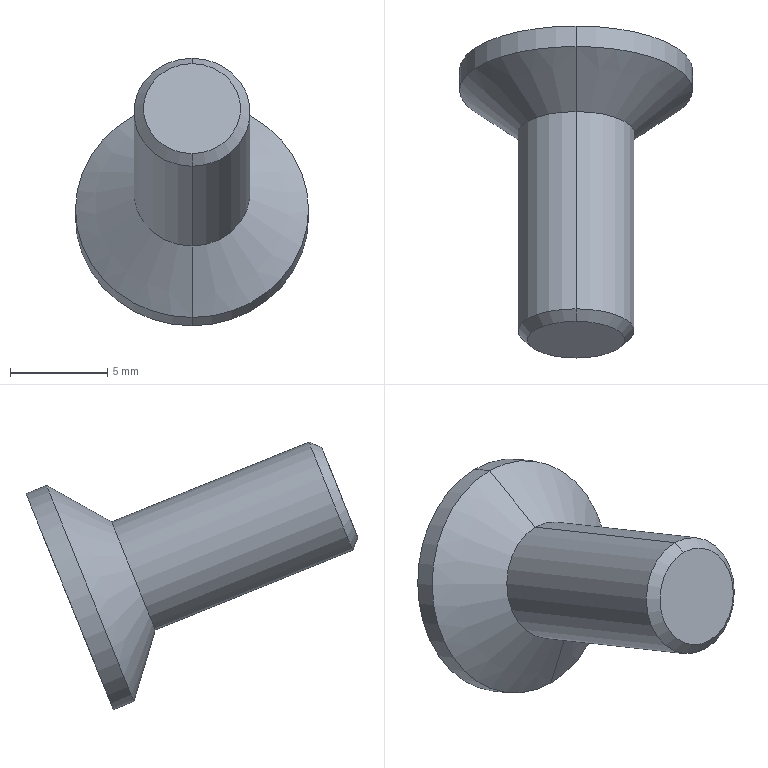Part | Creo | 1 solid | 18 faces | box 12 x 17.092 x 13.776 mm | volume 560.254 mm3 | plane 8 | cone 6 | cylinder 4 | commonest cylinder face diameters 6 x2 12 x2
STEP:
#1=CARTESIAN_POINT('',(50.258,-269.39,4.596));
#2=VERTEX_POINT('',#1);
#3=CARTESIAN_POINT('',(52.258,-269.822,3.525));
#4=VERTEX_POINT('',#3);
#5=CARTESIAN_POINT('',(50.258,-269.39,4.596));
#6=CARTESIAN_POINT('',(50.351,-269.439,4.558));
#7=CARTESIAN_POINT('',(50.539,-269.531,4.479));
#8=CARTESIAN_POINT('',(50.825,-269.649,4.348));
#9=CARTESIAN_POINT('',(51.114,-269.742,4.205));
#10=CARTESIAN_POINT('',(51.404,-269.804,4.05));
#11=CARTESIAN_POINT('',(51.693,-269.837,3.883));
#12=CARTESIAN_POINT('',(51.979,-269.842,3.707));
#13=CARTESIAN_POINT('',(52.166,-269.831,3.587));
#14=CARTESIAN_POINT('',(52.258,-269.822,3.525));
#15=B_SPLINE_CURVE_WITH_KNOTS('',3,(#5,#6,#7,#8,#9,#10,#11,#12,#13,#14),.UNSPECIFIED.,.F.,.F.,(4,1,1,1,1,1,1,4),(0.,0.1429,0.2857,0.4286,0.5714,0.7143,0.8571,1.),.UNSPECIFIED.);
#16=EDGE_CURVE('',#2,#4,#15,.T.);
#17=ORIENTED_EDGE('',*,*,#16,.F.);
#18=CARTESIAN_POINT('',(50.258,-271.491,2.954));
#19=VERTEX_POINT('',#18);
#20=CARTESIAN_POINT('',(50.258,-271.491,2.954));
#21=DIRECTION('',(0.,0.788,0.6157));
#22=VECTOR('',#21,2.667);
#23=LINE('',#20,#22);
#24=EDGE_CURVE('',#19,#2,#23,.T.);
#25=ORIENTED_EDGE('',*,*,#24,.F.);
#26=CARTESIAN_POINT('',(50.258,-271.12,0.3135));
#27=VERTEX_POINT('',#26);
#28=CARTESIAN_POINT('',(50.258,-271.491,2.954));
#29=DIRECTION('',(0.,0.1392,-0.9903));
#30=VECTOR('',#29,2.667);
#31=LINE('',#28,#30);
#32=EDGE_CURVE('',#19,#27,#31,.T.);
#33=ORIENTED_EDGE('',*,*,#32,.T.);
#34=CARTESIAN_POINT('',(52.258,-270.687,1.384));
#35=VERTEX_POINT('',#34);
#36=CARTESIAN_POINT('',(52.258,-270.687,1.384));
#37=CARTESIAN_POINT('',(52.166,-270.736,1.346));
#38=CARTESIAN_POINT('',(51.979,-270.828,1.267));
#39=CARTESIAN_POINT('',(51.693,-270.947,1.137));
#40=CARTESIAN_POINT('',(51.404,-271.039,0.9941));
#41=CARTESIAN_POINT('',(51.114,-271.102,0.8392));
#42=CARTESIAN_POINT('',(50.825,-271.134,0.6724));
#43=CARTESIAN_POINT('',(50.539,-271.14,0.4961));
#44=CARTESIAN_POINT('',(50.351,-271.129,0.375));
#45=CARTESIAN_POINT('',(50.258,-271.12,0.3135));
#46=B_SPLINE_CURVE_WITH_KNOTS('',3,(#36,#37,#38,#39,#40,#41,#42,#43,#44,#45),.UNSPECIFIED.,.F.,.F.,(4,1,1,1,1,1,1,4),(0.,0.1429,0.2857,0.4286,0.5714,0.7143,0.8571,1.),.UNSPECIFIED.);
#47=EDGE_CURVE('',#35,#27,#46,.T.);
#48=ORIENTED_EDGE('',*,*,#47,.F.);
#49=CARTESIAN_POINT('',(52.258,-269.822,3.525));
#50=CARTESIAN_POINT('',(52.258,-269.862,3.474));
#51=CARTESIAN_POINT('',(52.258,-269.939,3.373));
#52=CARTESIAN_POINT('',(52.258,-270.044,3.224));
#53=CARTESIAN_POINT('',(52.258,-270.14,3.075));
#54=CARTESIAN_POINT('',(52.258,-270.229,2.924));
#55=CARTESIAN_POINT('',(52.258,-270.312,2.767));
#56=CARTESIAN_POINT('',(52.258,-270.387,2.605));
#57=CARTESIAN_POINT('',(52.258,-270.454,2.439));
#58=CARTESIAN_POINT('',(52.258,-270.513,2.27));
#59=CARTESIAN_POINT('',(52.258,-270.562,2.1));
#60=CARTESIAN_POINT('',(52.258,-270.603,1.928));
#61=CARTESIAN_POINT('',(52.258,-270.637,1.754));
#62=CARTESIAN_POINT('',(52.258,-270.665,1.575));
#63=CARTESIAN_POINT('',(52.258,-270.681,1.449));
#64=CARTESIAN_POINT('',(52.258,-270.687,1.384));
#65=B_SPLINE_CURVE_WITH_KNOTS('',3,(#49,#50,#51,#52,#53,#54,#55,#56,#57,#58,#59,#60,#61,#62,#63,#64),.UNSPECIFIED.,.F.,.F.,(4,1,1,1,1,1,1,1,1,1,1,1,1,4),(0.,0.07692,0.1538,0.2308,0.3077,0.3846,0.4615,0.5385,0.6154,0.6923,0.7692,0.8462,0.9231,1.),.UNSPECIFIED.);
#66=EDGE_CURVE('',#4,#35,#65,.T.);
#67=ORIENTED_EDGE('',*,*,#66,.F.);
#68=EDGE_LOOP('',(#17,#25,#33,#48,#67));
#69=FACE_OUTER_BOUND('',#68,.F.);
#70=CARTESIAN_POINT('',(50.258,-270.861,2.699));
#71=DIRECTION('',(0.,0.9272,-0.3746));
#72=DIRECTION('',(0.,0.3746,0.9272));
#73=AXIS2_PLACEMENT_3D('',#70,#71,#72);
#74=CONICAL_SURFACE('',#73,1.178,60.);
#75=ADVANCED_FACE('',(#69),#74,.F.);
#76=CARTESIAN_POINT('',(52.258,-267.041,2.402));
#77=VERTEX_POINT('',#76);
#78=CARTESIAN_POINT('',(50.258,-266.608,3.472));
#79=VERTEX_POINT('',#78);
#80=CARTESIAN_POINT('',(52.258,-267.041,2.402));
#81=DIRECTION('',(-0.866,0.1873,0.4636));
#82=VECTOR('',#81,2.309);
#83=LINE('',#80,#82);
#84=EDGE_CURVE('',#77,#79,#83,.T.);
#85=ORIENTED_EDGE('',*,*,#84,.T.);
#86=CARTESIAN_POINT('',(50.258,-266.608,3.472));
#87=DIRECTION('',(0.,-0.9272,0.3746));
#88=VECTOR('',#87,3.);
#89=LINE('',#86,#88);
#90=EDGE_CURVE('',#79,#2,#89,.T.);
#91=ORIENTED_EDGE('',*,*,#90,.T.);
#92=ORIENTED_EDGE('',*,*,#16,.T.);
#93=CARTESIAN_POINT('',(52.258,-267.041,2.402));
#94=DIRECTION('',(0.,-0.9272,0.3746));
#95=VECTOR('',#94,3.);
#96=LINE('',#93,#95);
#97=EDGE_CURVE('',#77,#4,#96,.T.);
#98=ORIENTED_EDGE('',*,*,#97,.F.);
#99=EDGE_LOOP('',(#85,#91,#92,#98));
#100=FACE_OUTER_BOUND('',#99,.F.);
#101=CARTESIAN_POINT('',(50.258,-269.39,4.596));
#102=DIRECTION('',(0.5,0.3244,0.803));
#103=DIRECTION('',(0.866,-0.1873,-0.4636));
#104=AXIS2_PLACEMENT_3D('',#101,#102,#103);
#105=PLANE('',#104);
#106=ADVANCED_FACE('',(#100),#105,.F.);
#107=CARTESIAN_POINT('',(50.258,-265.226,6.894));
#108=VERTEX_POINT('',#107);
#109=CARTESIAN_POINT('',(50.258,-269.721,-4.232));
#110=VERTEX_POINT('',#109);
#111=CARTESIAN_POINT('',(50.258,-267.473,1.331));
#112=DIRECTION('',(0.,0.9272,-0.3746));
#113=DIRECTION('',(0.,0.3746,0.9272));
#114=AXIS2_PLACEMENT_3D('',#111,#112,#113);
#115=CIRCLE('',#114,6.);
#116=EDGE_CURVE('',#108,#110,#115,.T.);
#117=ORIENTED_EDGE('',*,*,#116,.F.);
#118=CARTESIAN_POINT('',(50.258,-267.473,1.331));
#119=DIRECTION('',(0.,0.9272,-0.3746));
#120=DIRECTION('',(0.,-0.3746,-0.9272));
#121=AXIS2_PLACEMENT_3D('',#118,#119,#120);
#122=CIRCLE('',#121,6.);
#123=EDGE_CURVE('',#110,#108,#122,.T.);
#124=ORIENTED_EDGE('',*,*,#123,.F.);
#125=EDGE_LOOP('',(#117,#124));
#126=FACE_OUTER_BOUND('',#125,.F.);
#127=CARTESIAN_POINT('',(52.258,-267.906,0.2603));
#128=VERTEX_POINT('',#127);
#129=CARTESIAN_POINT('',(52.258,-267.906,0.2603));
#130=DIRECTION('',(0.,0.3746,0.9272));
#131=VECTOR('',#130,2.309);
#132=LINE('',#129,#131);
#133=EDGE_CURVE('',#128,#77,#132,.T.);
#134=ORIENTED_EDGE('',*,*,#133,.F.);
#135=CARTESIAN_POINT('',(50.258,-268.338,-0.8103));
#136=VERTEX_POINT('',#135);
#137=CARTESIAN_POINT('',(50.258,-268.338,-0.8103));
#138=DIRECTION('',(0.866,0.1873,0.4636));
#139=VECTOR('',#138,2.309);
#140=LINE('',#137,#139);
#141=EDGE_CURVE('',#136,#128,#140,.T.);
#142=ORIENTED_EDGE('',*,*,#141,.F.);
#143=CARTESIAN_POINT('',(48.258,-267.906,0.2603));
#144=VERTEX_POINT('',#143);
#145=CARTESIAN_POINT('',(48.258,-267.906,0.2603));
#146=DIRECTION('',(0.866,-0.1873,-0.4636));
#147=VECTOR('',#146,2.309);
#148=LINE('',#145,#147);
#149=EDGE_CURVE('',#144,#136,#148,.T.);
#150=ORIENTED_EDGE('',*,*,#149,.F.);
#151=CARTESIAN_POINT('',(48.258,-267.041,2.402));
#152=VERTEX_POINT('',#151);
#153=CARTESIAN_POINT('',(48.258,-267.041,2.402));
#154=DIRECTION('',(0.,-0.3746,-0.9272));
#155=VECTOR('',#154,2.309);
#156=LINE('',#153,#155);
#157=EDGE_CURVE('',#152,#144,#156,.T.);
#158=ORIENTED_EDGE('',*,*,#157,.F.);
#159=CARTESIAN_POINT('',(50.258,-266.608,3.472));
#160=DIRECTION('',(-0.866,-0.1873,-0.4636));
#161=VECTOR('',#160,2.309);
#162=LINE('',#159,#161);
#163=EDGE_CURVE('',#79,#152,#162,.T.);
#164=ORIENTED_EDGE('',*,*,#163,.F.);
#165=ORIENTED_EDGE('',*,*,#84,.F.);
#166=EDGE_LOOP('',(#134,#142,#150,#158,#164,#165));
#167=FACE_BOUND('',#166,.F.);
#168=CARTESIAN_POINT('',(50.258,-265.226,6.894));
#169=DIRECTION('',(0.,-0.9272,0.3746));
#170=DIRECTION('',(0.,-0.3746,-0.9272));
#171=AXIS2_PLACEMENT_3D('',#168,#169,#170);
#172=PLANE('',#171);
#173=ADVANCED_FACE('',(#126,#167),#172,.F.);
#174=ORIENTED_EDGE('',*,*,#133,.T.);
#175=ORIENTED_EDGE('',*,*,#97,.T.);
#176=ORIENTED_EDGE('',*,*,#66,.T.);
#177=CARTESIAN_POINT('',(52.258,-267.906,0.2603));
#178=DIRECTION('',(0.,-0.9272,0.3746));
#179=VECTOR('',#178,3.);
#180=LINE('',#177,#179);
#181=EDGE_CURVE('',#128,#35,#180,.T.);
#182=ORIENTED_EDGE('',*,*,#181,.F.);
#183=EDGE_LOOP('',(#174,#175,#176,#182));
#184=FACE_OUTER_BOUND('',#183,.F.);
#185=CARTESIAN_POINT('',(52.258,-269.822,3.525));
#186=DIRECTION('',(1.,0.,0.));
#187=DIRECTION('',(0.,0.9272,-0.3746));
#188=AXIS2_PLACEMENT_3D('',#185,#186,#187);
#189=PLANE('',#188);
#190=ADVANCED_FACE('',(#184),#189,.F.);
#191=ORIENTED_EDGE('',*,*,#141,.T.);
#192=ORIENTED_EDGE('',*,*,#181,.T.);
#193=ORIENTED_EDGE('',*,*,#47,.T.);
#194=CARTESIAN_POINT('',(50.258,-268.338,-0.8103));
#195=DIRECTION('',(0.,-0.9272,0.3746));
#196=VECTOR('',#195,3.);
#197=LINE('',#194,#196);
#198=EDGE_CURVE('',#136,#27,#197,.T.);
#199=ORIENTED_EDGE('',*,*,#198,.F.);
#200=EDGE_LOOP('',(#191,#192,#193,#199));
#201=FACE_OUTER_BOUND('',#200,.F.);
#202=CARTESIAN_POINT('',(52.258,-270.687,1.384));
#203=DIRECTION('',(0.5,-0.3244,-0.803));
#204=DIRECTION('',(-0.866,-0.1873,-0.4636));
#205=AXIS2_PLACEMENT_3D('',#202,#203,#204);
#206=PLANE('',#205);
#207=ADVANCED_FACE('',(#201),#206,.F.);
#208=ORIENTED_EDGE('',*,*,#149,.T.);
#209=ORIENTED_EDGE('',*,*,#198,.T.);
#210=CARTESIAN_POINT('',(48.258,-270.687,1.384));
#211=VERTEX_POINT('',#210);
#212=CARTESIAN_POINT('',(50.258,-271.12,0.3135));
#213=CARTESIAN_POINT('',(50.165,-271.129,0.375));
#214=CARTESIAN_POINT('',(49.978,-271.14,0.4961));
#215=CARTESIAN_POINT('',(49.692,-271.134,0.6724));
#216=CARTESIAN_POINT('',(49.402,-271.102,0.8392));
#217=CARTESIAN_POINT('',(49.113,-271.039,0.9941));
#218=CARTESIAN_POINT('',(48.824,-270.947,1.137));
#219=CARTESIAN_POINT('',(48.538,-270.828,1.267));
#220=CARTESIAN_POINT('',(48.351,-270.736,1.346));
#221=CARTESIAN_POINT('',(48.258,-270.687,1.384));
#222=B_SPLINE_CURVE_WITH_KNOTS('',3,(#212,#213,#214,#215,#216,#217,#218,#219,#220,#221),.UNSPECIFIED.,.F.,.F.,(4,1,1,1,1,1,1,4),(0.,0.1429,0.2857,0.4286,0.5714,0.7143,0.8571,1.),.UNSPECIFIED.);
#223=EDGE_CURVE('',#27,#211,#222,.T.);
#224=ORIENTED_EDGE('',*,*,#223,.T.);
#225=CARTESIAN_POINT('',(48.258,-267.906,0.2603));
#226=DIRECTION('',(0.,-0.9272,0.3746));
#227=VECTOR('',#226,3.);
#228=LINE('',#225,#227);
#229=EDGE_CURVE('',#144,#211,#228,.T.);
#230=ORIENTED_EDGE('',*,*,#229,.F.);
#231=EDGE_LOOP('',(#208,#209,#224,#230));
#232=FACE_OUTER_BOUND('',#231,.F.);
#233=CARTESIAN_POINT('',(50.258,-271.12,0.3135));
#234=DIRECTION('',(-0.5,-0.3244,-0.803));
#235=DIRECTION('',(-0.866,0.1873,0.4636));
#236=AXIS2_PLACEMENT_3D('',#233,#234,#235);
#237=PLANE('',#236);
#238=ADVANCED_FACE('',(#232),#237,.F.);
#239=CARTESIAN_POINT('',(48.258,-269.822,3.525));
#240=VERTEX_POINT('',#239);
#241=CARTESIAN_POINT('',(48.258,-270.687,1.384));
#242=CARTESIAN_POINT('',(48.258,-270.681,1.449));
#243=CARTESIAN_POINT('',(48.258,-270.665,1.575));
#244=CARTESIAN_POINT('',(48.258,-270.637,1.754));
#245=CARTESIAN_POINT('',(48.258,-270.603,1.928));
#246=CARTESIAN_POINT('',(48.258,-270.562,2.1));
#247=CARTESIAN_POINT('',(48.258,-270.513,2.27));
#248=CARTESIAN_POINT('',(48.258,-270.454,2.439));
#249=CARTESIAN_POINT('',(48.258,-270.387,2.605));
#250=CARTESIAN_POINT('',(48.258,-270.312,2.767));
#251=CARTESIAN_POINT('',(48.258,-270.229,2.924));
#252=CARTESIAN_POINT('',(48.258,-270.14,3.075));
#253=CARTESIAN_POINT('',(48.258,-270.044,3.224));
#254=CARTESIAN_POINT('',(48.258,-269.939,3.373));
#255=CARTESIAN_POINT('',(48.258,-269.862,3.474));
#256=CARTESIAN_POINT('',(48.258,-269.822,3.525));
#257=B_SPLINE_CURVE_WITH_KNOTS('',3,(#241,#242,#243,#244,#245,#246,#247,#248,#249,#250,#251,#252,#253,#254,#255,#256),.UNSPECIFIED.,.F.,.F.,(4,1,1,1,1,1,1,1,1,1,1,1,1,4),(0.,0.07692,0.1538,0.2308,0.3077,0.3846,0.4615,0.5385,0.6154,0.6923,0.7692,0.8462,0.9231,1.),.UNSPECIFIED.);
#258=EDGE_CURVE('',#211,#240,#257,.T.);
#259=ORIENTED_EDGE('',*,*,#258,.F.);
#260=ORIENTED_EDGE('',*,*,#223,.F.);
#261=ORIENTED_EDGE('',*,*,#32,.F.);
#262=ORIENTED_EDGE('',*,*,#24,.T.);
#263=CARTESIAN_POINT('',(48.258,-269.822,3.525));
#264=CARTESIAN_POINT('',(48.351,-269.831,3.587));
#265=CARTESIAN_POINT('',(48.538,-269.842,3.707));
#266=CARTESIAN_POINT('',(48.824,-269.837,3.883));
#267=CARTESIAN_POINT('',(49.113,-269.804,4.05));
#268=CARTESIAN_POINT('',(49.402,-269.742,4.205));
#269=CARTESIAN_POINT('',(49.692,-269.649,4.348));
#270=CARTESIAN_POINT('',(49.978,-269.531,4.479));
#271=CARTESIAN_POINT('',(50.165,-269.439,4.558));
#272=CARTESIAN_POINT('',(50.258,-269.39,4.596));
#273=B_SPLINE_CURVE_WITH_KNOTS('',3,(#263,#264,#265,#266,#267,#268,#269,#270,#271,#272),.UNSPECIFIED.,.F.,.F.,(4,1,1,1,1,1,1,4),(0.,0.1429,0.2857,0.4286,0.5714,0.7143,0.8571,1.),.UNSPECIFIED.);
#274=EDGE_CURVE('',#240,#2,#273,.T.);
#275=ORIENTED_EDGE('',*,*,#274,.F.);
#276=EDGE_LOOP('',(#259,#260,#261,#262,#275));
#277=FACE_OUTER_BOUND('',#276,.F.);
#278=CARTESIAN_POINT('',(50.258,-270.861,2.699));
#279=DIRECTION('',(0.,0.9272,-0.3746));
#280=DIRECTION('',(0.,0.3746,0.9272));
#281=AXIS2_PLACEMENT_3D('',#278,#279,#280);
#282=CONICAL_SURFACE('',#281,1.178,60.);
#283=ADVANCED_FACE('',(#277),#282,.F.);
#284=ORIENTED_EDGE('',*,*,#157,.T.);
#285=ORIENTED_EDGE('',*,*,#229,.T.);
#286=ORIENTED_EDGE('',*,*,#258,.T.);
#287=CARTESIAN_POINT('',(48.258,-267.041,2.402));
#288=DIRECTION('',(0.,-0.9272,0.3746));
#289=VECTOR('',#288,3.);
#290=LINE('',#287,#289);
#291=EDGE_CURVE('',#152,#240,#290,.T.);
#292=ORIENTED_EDGE('',*,*,#291,.F.);
#293=EDGE_LOOP('',(#284,#285,#286,#292));
#294=FACE_OUTER_BOUND('',#293,.F.);
#295=CARTESIAN_POINT('',(48.258,-270.687,1.384));
#296=DIRECTION('',(-1.,0.,0.));
#297=DIRECTION('',(0.,-0.9272,0.3746));
#298=AXIS2_PLACEMENT_3D('',#295,#296,#297);
#299=PLANE('',#298);
#300=ADVANCED_FACE('',(#294),#299,.F.);
#301=ORIENTED_EDGE('',*,*,#163,.T.);
#302=ORIENTED_EDGE('',*,*,#291,.T.);
#303=ORIENTED_EDGE('',*,*,#274,.T.);
#304=ORIENTED_EDGE('',*,*,#90,.F.);
#305=EDGE_LOOP('',(#301,#302,#303,#304));
#306=FACE_OUTER_BOUND('',#305,.F.);
#307=CARTESIAN_POINT('',(48.258,-269.822,3.525));
#308=DIRECTION('',(-0.5,0.3244,0.803));
#309=DIRECTION('',(0.866,0.1873,0.4636));
#310=AXIS2_PLACEMENT_3D('',#307,#308,#309);
#311=PLANE('',#310);
#312=ADVANCED_FACE('',(#306),#311,.F.);
#313=ORIENTED_EDGE('',*,*,#116,.T.);
#314=CARTESIAN_POINT('',(50.258,-270.778,-3.805));
#315=VERTEX_POINT('',#314);
#316=CARTESIAN_POINT('',(50.258,-270.778,-3.805));
#317=DIRECTION('',(0.,0.9272,-0.3746));
#318=VECTOR('',#317,1.14);
#319=LINE('',#316,#318);
#320=EDGE_CURVE('',#315,#110,#319,.T.);
#321=ORIENTED_EDGE('',*,*,#320,.F.);
#322=CARTESIAN_POINT('',(50.258,-266.283,7.321));
#323=VERTEX_POINT('',#322);
#324=CARTESIAN_POINT('',(50.258,-268.53,1.758));
#325=DIRECTION('',(0.,-0.9272,0.3746));
#326=DIRECTION('',(0.,-0.3746,-0.9272));
#327=AXIS2_PLACEMENT_3D('',#324,#325,#326);
#328=CIRCLE('',#327,6.);
#329=EDGE_CURVE('',#315,#323,#328,.T.);
#330=ORIENTED_EDGE('',*,*,#329,.T.);
#331=CARTESIAN_POINT('',(50.258,-266.283,7.321));
#332=DIRECTION('',(0.,0.9272,-0.3746));
#333=VECTOR('',#332,1.14);
#334=LINE('',#331,#333);
#335=EDGE_CURVE('',#323,#108,#334,.T.);
#336=ORIENTED_EDGE('',*,*,#335,.T.);
#337=EDGE_LOOP('',(#313,#321,#330,#336));
#338=FACE_OUTER_BOUND('',#337,.F.);
#339=CARTESIAN_POINT('',(50.258,-266.546,0.9563));
#340=DIRECTION('',(0.,0.9272,-0.3746));
#341=DIRECTION('',(0.,0.3746,0.9272));
#342=AXIS2_PLACEMENT_3D('',#339,#340,#341);
#343=CYLINDRICAL_SURFACE('',#342,6.);
#344=ADVANCED_FACE('',(#338),#343,.T.);
#345=ORIENTED_EDGE('',*,*,#123,.T.);
#346=ORIENTED_EDGE('',*,*,#335,.F.);
#347=CARTESIAN_POINT('',(50.258,-268.53,1.758));
#348=DIRECTION('',(0.,-0.9272,0.3746));
#349=DIRECTION('',(0.,0.3746,0.9272));
#350=AXIS2_PLACEMENT_3D('',#347,#348,#349);
#351=CIRCLE('',#350,6.);
#352=EDGE_CURVE('',#323,#315,#351,.T.);
#353=ORIENTED_EDGE('',*,*,#352,.T.);
#354=ORIENTED_EDGE('',*,*,#320,.T.);
#355=EDGE_LOOP('',(#345,#346,#353,#354));
#356=FACE_OUTER_BOUND('',#355,.F.);
#357=CARTESIAN_POINT('',(50.258,-266.546,0.9563));
#358=DIRECTION('',(0.,0.9272,-0.3746));
#359=DIRECTION('',(0.,0.3746,0.9272));
#360=AXIS2_PLACEMENT_3D('',#357,#358,#359);
#361=CYLINDRICAL_SURFACE('',#360,6.);
#362=ADVANCED_FACE('',(#356),#361,.T.);
#363=CARTESIAN_POINT('',(50.258,-271.879,-0.1245));
#364=VERTEX_POINT('',#363);
#365=CARTESIAN_POINT('',(50.258,-269.632,5.439));
#366=VERTEX_POINT('',#365);
#367=CARTESIAN_POINT('',(50.258,-270.755,2.657));
#368=DIRECTION('',(0.,0.9272,-0.3746));
#369=DIRECTION('',(0.,-0.3746,-0.9272));
#370=AXIS2_PLACEMENT_3D('',#367,#368,#369);
#371=CIRCLE('',#370,3.);
#372=EDGE_CURVE('',#364,#366,#371,.T.);
#373=ORIENTED_EDGE('',*,*,#372,.F.);
#374=CARTESIAN_POINT('',(50.258,-271.879,-0.1245));
#375=DIRECTION('',(0.,0.2867,-0.958));
#376=VECTOR('',#375,3.842);
#377=LINE('',#374,#376);
#378=EDGE_CURVE('',#364,#315,#377,.T.);
#379=ORIENTED_EDGE('',*,*,#378,.T.);
#380=ORIENTED_EDGE('',*,*,#352,.F.);
#381=CARTESIAN_POINT('',(50.258,-269.632,5.439));
#382=DIRECTION('',(0.,0.8717,0.49));
#383=VECTOR('',#382,3.842);
#384=LINE('',#381,#383);
#385=EDGE_CURVE('',#366,#323,#384,.T.);
#386=ORIENTED_EDGE('',*,*,#385,.F.);
#387=EDGE_LOOP('',(#373,#379,#380,#386));
#388=FACE_OUTER_BOUND('',#387,.F.);
#389=CARTESIAN_POINT('',(50.258,-269.643,2.208));
#390=DIRECTION('',(0.,0.9272,-0.3746));
#391=DIRECTION('',(0.,0.3746,0.9272));
#392=AXIS2_PLACEMENT_3D('',#389,#390,#391);
#393=CONICAL_SURFACE('',#392,4.5,51.34);
#394=ADVANCED_FACE('',(#388),#393,.T.);
#395=ORIENTED_EDGE('',*,*,#372,.T.);
#396=CARTESIAN_POINT('',(50.258,-279.794,9.544));
#397=VERTEX_POINT('',#396);
#398=CARTESIAN_POINT('',(50.258,-279.794,9.544));
#399=DIRECTION('',(0.,0.9272,-0.3746));
#400=VECTOR('',#399,10.96);
#401=LINE('',#398,#400);
#402=EDGE_CURVE('',#397,#366,#401,.T.);
#403=ORIENTED_EDGE('',*,*,#402,.F.);
#404=CARTESIAN_POINT('',(50.258,-282.041,3.981));
#405=VERTEX_POINT('',#404);
#406=CARTESIAN_POINT('',(50.258,-280.917,6.763));
#407=DIRECTION('',(0.,-0.9272,0.3746));
#408=DIRECTION('',(0.,0.3746,0.9272));
#409=AXIS2_PLACEMENT_3D('',#406,#407,#408);
#410=CIRCLE('',#409,3.);
#411=EDGE_CURVE('',#397,#405,#410,.T.);
#412=ORIENTED_EDGE('',*,*,#411,.T.);
#413=CARTESIAN_POINT('',(50.258,-282.041,3.981));
#414=DIRECTION('',(0.,0.9272,-0.3746));
#415=VECTOR('',#414,10.96);
#416=LINE('',#413,#415);
#417=EDGE_CURVE('',#405,#364,#416,.T.);
#418=ORIENTED_EDGE('',*,*,#417,.T.);
#419=EDGE_LOOP('',(#395,#403,#412,#418));
#420=FACE_OUTER_BOUND('',#419,.F.);
#421=CARTESIAN_POINT('',(50.258,-266.546,0.9563));
#422=DIRECTION('',(0.,0.9272,-0.3746));
#423=DIRECTION('',(0.,0.3746,0.9272));
#424=AXIS2_PLACEMENT_3D('',#421,#422,#423);
#425=CYLINDRICAL_SURFACE('',#424,3.);
#426=ADVANCED_FACE('',(#420),#425,.T.);
#427=CARTESIAN_POINT('',(50.258,-270.755,2.657));
#428=DIRECTION('',(0.,0.9272,-0.3746));
#429=DIRECTION('',(0.,0.3746,0.9272));
#430=AXIS2_PLACEMENT_3D('',#427,#428,#429);
#431=CIRCLE('',#430,3.);
#432=EDGE_CURVE('',#366,#364,#431,.T.);
#433=ORIENTED_EDGE('',*,*,#432,.T.);
#434=ORIENTED_EDGE('',*,*,#417,.F.);
#435=CARTESIAN_POINT('',(50.258,-280.917,6.763));
#436=DIRECTION('',(0.,-0.9272,0.3746));
#437=DIRECTION('',(0.,-0.3746,-0.9272));
#438=AXIS2_PLACEMENT_3D('',#435,#436,#437);
#439=CIRCLE('',#438,3.);
#440=EDGE_CURVE('',#405,#397,#439,.T.);
#441=ORIENTED_EDGE('',*,*,#440,.T.);
#442=ORIENTED_EDGE('',*,*,#402,.T.);
#443=EDGE_LOOP('',(#433,#434,#441,#442));
#444=FACE_OUTER_BOUND('',#443,.F.);
#445=CARTESIAN_POINT('',(50.258,-266.546,0.9563));
#446=DIRECTION('',(0.,0.9272,-0.3746));
#447=DIRECTION('',(0.,0.3746,0.9272));
#448=AXIS2_PLACEMENT_3D('',#445,#446,#447);
#449=CYLINDRICAL_SURFACE('',#448,3.);
#450=ADVANCED_FACE('',(#444),#449,.T.);
#451=ORIENTED_EDGE('',*,*,#432,.F.);
#452=ORIENTED_EDGE('',*,*,#385,.T.);
#453=ORIENTED_EDGE('',*,*,#329,.F.);
#454=ORIENTED_EDGE('',*,*,#378,.F.);
#455=EDGE_LOOP('',(#451,#452,#453,#454));
#456=FACE_OUTER_BOUND('',#455,.F.);
#457=CARTESIAN_POINT('',(50.258,-269.643,2.208));
#458=DIRECTION('',(0.,0.9272,-0.3746));
#459=DIRECTION('',(0.,0.3746,0.9272));
#460=AXIS2_PLACEMENT_3D('',#457,#458,#459);
#461=CONICAL_SURFACE('',#460,4.5,51.34);
#462=ADVANCED_FACE('',(#456),#461,.T.);
#463=ORIENTED_EDGE('',*,*,#440,.F.);
#464=CARTESIAN_POINT('',(50.258,-282.317,4.632));
#465=VERTEX_POINT('',#464);
#466=CARTESIAN_POINT('',(50.258,-282.317,4.632));
#467=DIRECTION('',(0.,0.3907,-0.9205));
#468=VECTOR('',#467,0.7071);
#469=LINE('',#466,#468);
#470=EDGE_CURVE('',#465,#405,#469,.T.);
#471=ORIENTED_EDGE('',*,*,#470,.F.);
#472=CARTESIAN_POINT('',(50.258,-280.444,9.268));
#473=VERTEX_POINT('',#472);
#474=CARTESIAN_POINT('',(50.258,-281.381,6.95));
#475=DIRECTION('',(0.,-0.9272,0.3746));
#476=DIRECTION('',(0.,-0.3746,-0.9272));
#477=AXIS2_PLACEMENT_3D('',#474,#475,#476);
#478=CIRCLE('',#477,2.5);
#479=EDGE_CURVE('',#465,#473,#478,.T.);
#480=ORIENTED_EDGE('',*,*,#479,.T.);
#481=CARTESIAN_POINT('',(50.258,-280.444,9.268));
#482=DIRECTION('',(0.,0.9205,0.3907));
#483=VECTOR('',#482,0.7071);
#484=LINE('',#481,#483);
#485=EDGE_CURVE('',#473,#397,#484,.T.);
#486=ORIENTED_EDGE('',*,*,#485,.T.);
#487=EDGE_LOOP('',(#463,#471,#480,#486));
#488=FACE_OUTER_BOUND('',#487,.F.);
#489=CARTESIAN_POINT('',(50.258,-281.149,6.856));
#490=DIRECTION('',(0.,0.9272,-0.3746));
#491=DIRECTION('',(0.,0.3746,0.9272));
#492=AXIS2_PLACEMENT_3D('',#489,#490,#491);
#493=CONICAL_SURFACE('',#492,2.75,45.);
#494=ADVANCED_FACE('',(#488),#493,.T.);
#495=ORIENTED_EDGE('',*,*,#411,.F.);
#496=ORIENTED_EDGE('',*,*,#485,.F.);
#497=CARTESIAN_POINT('',(50.258,-281.381,6.95));
#498=DIRECTION('',(0.,-0.9272,0.3746));
#499=DIRECTION('',(0.,0.3746,0.9272));
#500=AXIS2_PLACEMENT_3D('',#497,#498,#499);
#501=CIRCLE('',#500,2.5);
#502=EDGE_CURVE('',#473,#465,#501,.T.);
#503=ORIENTED_EDGE('',*,*,#502,.T.);
#504=ORIENTED_EDGE('',*,*,#470,.T.);
#505=EDGE_LOOP('',(#495,#496,#503,#504));
#506=FACE_OUTER_BOUND('',#505,.F.);
#507=CARTESIAN_POINT('',(50.258,-281.149,6.856));
#508=DIRECTION('',(0.,0.9272,-0.3746));
#509=DIRECTION('',(0.,0.3746,0.9272));
#510=AXIS2_PLACEMENT_3D('',#507,#508,#509);
#511=CONICAL_SURFACE('',#510,2.75,45.);
#512=ADVANCED_FACE('',(#506),#511,.T.);
#513=ORIENTED_EDGE('',*,*,#502,.F.);
#514=ORIENTED_EDGE('',*,*,#479,.F.);
#515=EDGE_LOOP('',(#513,#514));
#516=FACE_OUTER_BOUND('',#515,.F.);
#517=CARTESIAN_POINT('',(50.258,-281.381,6.95));
#518=DIRECTION('',(0.,0.9272,-0.3746));
#519=DIRECTION('',(0.,0.3746,0.9272));
#520=AXIS2_PLACEMENT_3D('',#517,#518,#519);
#521=PLANE('',#520);
#522=ADVANCED_FACE('',(#516),#521,.F.);
#523=CLOSED_SHELL('',(#75,#106,#173,#190,#207,#238,#283,#300,#312,#344,#362,#394,#426,#450,#462,#494,#512,#522));
#524=MANIFOLD_SOLID_BREP('',#523);
#525=(LENGTH_UNIT()NAMED_UNIT(*)SI_UNIT(.MILLI.,.METRE.));
#526=UNCERTAINTY_MEASURE_WITH_UNIT(LENGTH_MEASURE(0.002502),#525,'','');
#527=(NAMED_UNIT(*)PLANE_ANGLE_UNIT()SI_UNIT($,.RADIAN.));
#528=PLANE_ANGLE_MEASURE_WITH_UNIT(PLANE_ANGLE_MEASURE(0.01745),#527);
#529=(CONVERSION_BASED_UNIT('DEGREE',#528)NAMED_UNIT(*)PLANE_ANGLE_UNIT());
#530=(NAMED_UNIT(*)SI_UNIT($,.STERADIAN.)SOLID_ANGLE_UNIT());
#531=(GEOMETRIC_REPRESENTATION_CONTEXT(3)GLOBAL_UNCERTAINTY_ASSIGNED_CONTEXT((#526))GLOBAL_UNIT_ASSIGNED_CONTEXT((#525,#529,#530))REPRESENTATION_CONTEXT('',''));
#532=ADVANCED_BREP_SHAPE_REPRESENTATION('',(#524),#531);